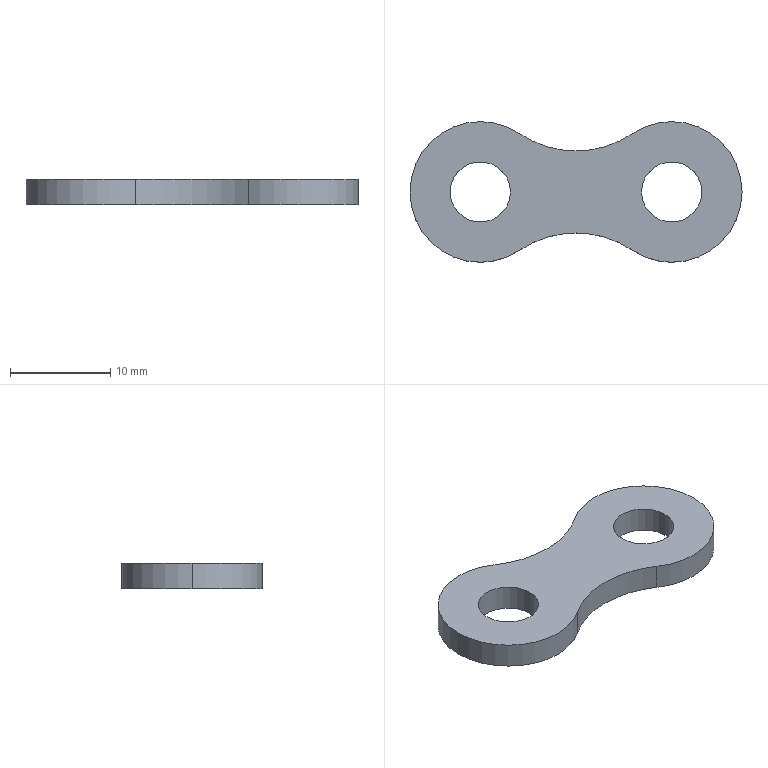Part | SolidWorks | features Extrusion 1 | 1 solid | 11 faces | box 33.05 x 14 x 2.55 mm | volume 777.67 mm3 | cylinder 9 | plane 2 | commonest cylinder face diameters 6 x4 14 x3 20 x2
STEP:
#1=CARTESIAN_POINT('',(16.05,0.,2.55));
#2=VERTEX_POINT('',#1);
#3=CARTESIAN_POINT('',(22.05,0.,2.55));
#4=VERTEX_POINT('',#3);
#5=CARTESIAN_POINT('',(19.05,0.,2.55));
#6=DIRECTION('',(0.,0.,1.));
#7=DIRECTION('',(1.,0.,0.));
#8=AXIS2_PLACEMENT_3D('',#5,#6,#7);
#9=CIRCLE('',#8,3.);
#10=EDGE_CURVE('',#2,#4,#9,.T.);
#11=ORIENTED_EDGE('',*,*,#10,.T.);
#12=CARTESIAN_POINT('',(22.05,0.,0.));
#13=VERTEX_POINT('',#12);
#14=CARTESIAN_POINT('',(22.05,0.,2.55));
#15=DIRECTION('',(0.,0.,-1.));
#16=VECTOR('',#15,1000.);
#17=LINE('',#14,#16);
#18=EDGE_CURVE('',#4,#13,#17,.T.);
#19=ORIENTED_EDGE('',*,*,#18,.T.);
#20=CARTESIAN_POINT('',(16.05,0.,0.));
#21=VERTEX_POINT('',#20);
#22=CARTESIAN_POINT('',(19.05,0.,0.));
#23=DIRECTION('',(0.,0.,1.));
#24=DIRECTION('',(1.,0.,0.));
#25=AXIS2_PLACEMENT_3D('',#22,#23,#24);
#26=CIRCLE('',#25,3.);
#27=EDGE_CURVE('',#21,#13,#26,.T.);
#28=ORIENTED_EDGE('',*,*,#27,.F.);
#29=CARTESIAN_POINT('',(16.05,0.,2.55));
#30=DIRECTION('',(0.,0.,-1.));
#31=VECTOR('',#30,1000.);
#32=LINE('',#29,#31);
#33=EDGE_CURVE('',#2,#21,#32,.T.);
#34=ORIENTED_EDGE('',*,*,#33,.F.);
#35=EDGE_LOOP('',(#11,#19,#28,#34));
#36=FACE_OUTER_BOUND('',#35,.T.);
#37=CARTESIAN_POINT('',(19.05,0.,2.55));
#38=DIRECTION('',(0.,0.,-1.));
#39=DIRECTION('',(-1.,0.,0.));
#40=AXIS2_PLACEMENT_3D('',#37,#38,#39);
#41=CYLINDRICAL_SURFACE('',#40,3.);
#42=ADVANCED_FACE('',(#36),#41,.F.);
#43=CARTESIAN_POINT('',(-3.,0.,2.55));
#44=VERTEX_POINT('',#43);
#45=CARTESIAN_POINT('',(3.,0.,2.55));
#46=VERTEX_POINT('',#45);
#47=CARTESIAN_POINT('',(0.,0.,2.55));
#48=DIRECTION('',(0.,0.,1.));
#49=DIRECTION('',(1.,0.,0.));
#50=AXIS2_PLACEMENT_3D('',#47,#48,#49);
#51=CIRCLE('',#50,3.);
#52=EDGE_CURVE('',#44,#46,#51,.T.);
#53=ORIENTED_EDGE('',*,*,#52,.T.);
#54=CARTESIAN_POINT('',(3.,0.,0.));
#55=VERTEX_POINT('',#54);
#56=CARTESIAN_POINT('',(3.,0.,2.55));
#57=DIRECTION('',(0.,0.,-1.));
#58=VECTOR('',#57,1000.);
#59=LINE('',#56,#58);
#60=EDGE_CURVE('',#46,#55,#59,.T.);
#61=ORIENTED_EDGE('',*,*,#60,.T.);
#62=CARTESIAN_POINT('',(-3.,0.,0.));
#63=VERTEX_POINT('',#62);
#64=CARTESIAN_POINT('',(0.,0.,0.));
#65=DIRECTION('',(0.,0.,1.));
#66=DIRECTION('',(1.,0.,0.));
#67=AXIS2_PLACEMENT_3D('',#64,#65,#66);
#68=CIRCLE('',#67,3.);
#69=EDGE_CURVE('',#63,#55,#68,.T.);
#70=ORIENTED_EDGE('',*,*,#69,.F.);
#71=CARTESIAN_POINT('',(-3.,0.,2.55));
#72=DIRECTION('',(0.,0.,-1.));
#73=VECTOR('',#72,1000.);
#74=LINE('',#71,#73);
#75=EDGE_CURVE('',#44,#63,#74,.T.);
#76=ORIENTED_EDGE('',*,*,#75,.F.);
#77=EDGE_LOOP('',(#53,#61,#70,#76));
#78=FACE_OUTER_BOUND('',#77,.T.);
#79=CARTESIAN_POINT('',(0.,0.,2.55));
#80=DIRECTION('',(0.,0.,-1.));
#81=DIRECTION('',(-1.,0.,0.));
#82=AXIS2_PLACEMENT_3D('',#79,#80,#81);
#83=CYLINDRICAL_SURFACE('',#82,3.);
#84=ADVANCED_FACE('',(#78),#83,.F.);
#85=CARTESIAN_POINT('',(-7.,0.,2.55));
#86=VERTEX_POINT('',#85);
#87=CARTESIAN_POINT('',(3.922,-5.798,2.55));
#88=VERTEX_POINT('',#87);
#89=CARTESIAN_POINT('',(0.,0.,2.55));
#90=DIRECTION('',(0.,0.,1.));
#91=DIRECTION('',(1.,0.,0.));
#92=AXIS2_PLACEMENT_3D('',#89,#90,#91);
#93=CIRCLE('',#92,7.);
#94=EDGE_CURVE('',#86,#88,#93,.T.);
#95=ORIENTED_EDGE('',*,*,#94,.F.);
#96=CARTESIAN_POINT('',(-7.,0.,0.));
#97=VERTEX_POINT('',#96);
#98=CARTESIAN_POINT('',(-7.,0.,2.55));
#99=DIRECTION('',(0.,0.,-1.));
#100=VECTOR('',#99,1000.);
#101=LINE('',#98,#100);
#102=EDGE_CURVE('',#86,#97,#101,.T.);
#103=ORIENTED_EDGE('',*,*,#102,.T.);
#104=CARTESIAN_POINT('',(3.922,-5.798,0.));
#105=VERTEX_POINT('',#104);
#106=CARTESIAN_POINT('',(0.,0.,0.));
#107=DIRECTION('',(0.,0.,1.));
#108=DIRECTION('',(1.,0.,0.));
#109=AXIS2_PLACEMENT_3D('',#106,#107,#108);
#110=CIRCLE('',#109,7.);
#111=EDGE_CURVE('',#97,#105,#110,.T.);
#112=ORIENTED_EDGE('',*,*,#111,.T.);
#113=CARTESIAN_POINT('',(3.922,-5.798,2.55));
#114=DIRECTION('',(0.,0.,-1.));
#115=VECTOR('',#114,1000.);
#116=LINE('',#113,#115);
#117=EDGE_CURVE('',#88,#105,#116,.T.);
#118=ORIENTED_EDGE('',*,*,#117,.F.);
#119=EDGE_LOOP('',(#95,#103,#112,#118));
#120=FACE_OUTER_BOUND('',#119,.T.);
#121=CARTESIAN_POINT('',(0.,0.,2.55));
#122=DIRECTION('',(0.,0.,-1.));
#123=DIRECTION('',(-1.,0.,0.));
#124=AXIS2_PLACEMENT_3D('',#121,#122,#123);
#125=CYLINDRICAL_SURFACE('',#124,7.);
#126=ADVANCED_FACE('',(#120),#125,.T.);
#127=ORIENTED_EDGE('',*,*,#52,.F.);
#128=CARTESIAN_POINT('',(0.,0.,2.55));
#129=DIRECTION('',(0.,0.,1.));
#130=DIRECTION('',(1.,0.,0.));
#131=AXIS2_PLACEMENT_3D('',#128,#129,#130);
#132=CIRCLE('',#131,3.);
#133=EDGE_CURVE('',#46,#44,#132,.T.);
#134=ORIENTED_EDGE('',*,*,#133,.F.);
#135=EDGE_LOOP('',(#127,#134));
#136=FACE_BOUND('',#135,.T.);
#137=CARTESIAN_POINT('',(15.128,5.798,2.55));
#138=VERTEX_POINT('',#137);
#139=CARTESIAN_POINT('',(3.922,5.798,2.55));
#140=VERTEX_POINT('',#139);
#141=CARTESIAN_POINT('',(9.525,14.081,2.55));
#142=DIRECTION('',(0.,0.,-1.));
#143=DIRECTION('',(1.,0.,0.));
#144=AXIS2_PLACEMENT_3D('',#141,#142,#143);
#145=CIRCLE('',#144,10.);
#146=EDGE_CURVE('',#138,#140,#145,.T.);
#147=ORIENTED_EDGE('',*,*,#146,.T.);
#148=CARTESIAN_POINT('',(0.,0.,2.55));
#149=DIRECTION('',(0.,0.,1.));
#150=DIRECTION('',(1.,0.,0.));
#151=AXIS2_PLACEMENT_3D('',#148,#149,#150);
#152=CIRCLE('',#151,7.);
#153=EDGE_CURVE('',#140,#86,#152,.T.);
#154=ORIENTED_EDGE('',*,*,#153,.T.);
#155=ORIENTED_EDGE('',*,*,#94,.T.);
#156=CARTESIAN_POINT('',(15.128,-5.798,2.55));
#157=VERTEX_POINT('',#156);
#158=CARTESIAN_POINT('',(9.525,-14.081,2.55));
#159=DIRECTION('',(0.,0.,-1.));
#160=DIRECTION('',(-1.,0.,0.));
#161=AXIS2_PLACEMENT_3D('',#158,#159,#160);
#162=CIRCLE('',#161,10.);
#163=EDGE_CURVE('',#88,#157,#162,.T.);
#164=ORIENTED_EDGE('',*,*,#163,.T.);
#165=CARTESIAN_POINT('',(19.05,0.,2.55));
#166=DIRECTION('',(0.,0.,1.));
#167=DIRECTION('',(1.,0.,0.));
#168=AXIS2_PLACEMENT_3D('',#165,#166,#167);
#169=CIRCLE('',#168,7.);
#170=EDGE_CURVE('',#157,#138,#169,.T.);
#171=ORIENTED_EDGE('',*,*,#170,.T.);
#172=EDGE_LOOP('',(#147,#154,#155,#164,#171));
#173=FACE_OUTER_BOUND('',#172,.T.);
#174=ORIENTED_EDGE('',*,*,#10,.F.);
#175=CARTESIAN_POINT('',(19.05,0.,2.55));
#176=DIRECTION('',(0.,0.,1.));
#177=DIRECTION('',(1.,0.,0.));
#178=AXIS2_PLACEMENT_3D('',#175,#176,#177);
#179=CIRCLE('',#178,3.);
#180=EDGE_CURVE('',#4,#2,#179,.T.);
#181=ORIENTED_EDGE('',*,*,#180,.F.);
#182=EDGE_LOOP('',(#174,#181));
#183=FACE_BOUND('',#182,.T.);
#184=CARTESIAN_POINT('',(14.288,7.04,2.55));
#185=DIRECTION('',(0.,0.,1.));
#186=DIRECTION('',(1.,0.,0.));
#187=AXIS2_PLACEMENT_3D('',#184,#185,#186);
#188=PLANE('',#187);
#189=ADVANCED_FACE('',(#136,#173,#183),#188,.T.);
#190=ORIENTED_EDGE('',*,*,#69,.T.);
#191=CARTESIAN_POINT('',(0.,0.,0.));
#192=DIRECTION('',(0.,0.,1.));
#193=DIRECTION('',(1.,0.,0.));
#194=AXIS2_PLACEMENT_3D('',#191,#192,#193);
#195=CIRCLE('',#194,3.);
#196=EDGE_CURVE('',#55,#63,#195,.T.);
#197=ORIENTED_EDGE('',*,*,#196,.T.);
#198=EDGE_LOOP('',(#190,#197));
#199=FACE_BOUND('',#198,.T.);
#200=CARTESIAN_POINT('',(15.128,5.798,0.));
#201=VERTEX_POINT('',#200);
#202=CARTESIAN_POINT('',(3.922,5.798,0.));
#203=VERTEX_POINT('',#202);
#204=CARTESIAN_POINT('',(9.525,14.081,0.));
#205=DIRECTION('',(0.,0.,-1.));
#206=DIRECTION('',(1.,0.,0.));
#207=AXIS2_PLACEMENT_3D('',#204,#205,#206);
#208=CIRCLE('',#207,10.);
#209=EDGE_CURVE('',#201,#203,#208,.T.);
#210=ORIENTED_EDGE('',*,*,#209,.F.);
#211=CARTESIAN_POINT('',(15.128,-5.798,0.));
#212=VERTEX_POINT('',#211);
#213=CARTESIAN_POINT('',(19.05,0.,0.));
#214=DIRECTION('',(0.,0.,1.));
#215=DIRECTION('',(1.,0.,0.));
#216=AXIS2_PLACEMENT_3D('',#213,#214,#215);
#217=CIRCLE('',#216,7.);
#218=EDGE_CURVE('',#212,#201,#217,.T.);
#219=ORIENTED_EDGE('',*,*,#218,.F.);
#220=CARTESIAN_POINT('',(9.525,-14.081,0.));
#221=DIRECTION('',(0.,0.,-1.));
#222=DIRECTION('',(-1.,0.,0.));
#223=AXIS2_PLACEMENT_3D('',#220,#221,#222);
#224=CIRCLE('',#223,10.);
#225=EDGE_CURVE('',#105,#212,#224,.T.);
#226=ORIENTED_EDGE('',*,*,#225,.F.);
#227=ORIENTED_EDGE('',*,*,#111,.F.);
#228=CARTESIAN_POINT('',(0.,0.,0.));
#229=DIRECTION('',(0.,0.,1.));
#230=DIRECTION('',(1.,0.,0.));
#231=AXIS2_PLACEMENT_3D('',#228,#229,#230);
#232=CIRCLE('',#231,7.);
#233=EDGE_CURVE('',#203,#97,#232,.T.);
#234=ORIENTED_EDGE('',*,*,#233,.F.);
#235=EDGE_LOOP('',(#210,#219,#226,#227,#234));
#236=FACE_OUTER_BOUND('',#235,.T.);
#237=ORIENTED_EDGE('',*,*,#27,.T.);
#238=CARTESIAN_POINT('',(19.05,0.,0.));
#239=DIRECTION('',(0.,0.,1.));
#240=DIRECTION('',(1.,0.,0.));
#241=AXIS2_PLACEMENT_3D('',#238,#239,#240);
#242=CIRCLE('',#241,3.);
#243=EDGE_CURVE('',#13,#21,#242,.T.);
#244=ORIENTED_EDGE('',*,*,#243,.T.);
#245=EDGE_LOOP('',(#237,#244));
#246=FACE_BOUND('',#245,.T.);
#247=CARTESIAN_POINT('',(14.288,7.04,0.));
#248=DIRECTION('',(0.,0.,1.));
#249=DIRECTION('',(1.,0.,0.));
#250=AXIS2_PLACEMENT_3D('',#247,#248,#249);
#251=PLANE('',#250);
#252=ADVANCED_FACE('',(#199,#236,#246),#251,.F.);
#253=ORIENTED_EDGE('',*,*,#209,.T.);
#254=CARTESIAN_POINT('',(3.922,5.798,2.55));
#255=DIRECTION('',(0.,0.,-1.));
#256=VECTOR('',#255,1000.);
#257=LINE('',#254,#256);
#258=EDGE_CURVE('',#140,#203,#257,.T.);
#259=ORIENTED_EDGE('',*,*,#258,.F.);
#260=ORIENTED_EDGE('',*,*,#146,.F.);
#261=CARTESIAN_POINT('',(15.128,5.798,2.55));
#262=DIRECTION('',(0.,0.,-1.));
#263=VECTOR('',#262,1000.);
#264=LINE('',#261,#263);
#265=EDGE_CURVE('',#138,#201,#264,.T.);
#266=ORIENTED_EDGE('',*,*,#265,.T.);
#267=EDGE_LOOP('',(#253,#259,#260,#266));
#268=FACE_OUTER_BOUND('',#267,.T.);
#269=CARTESIAN_POINT('',(9.525,14.081,2.55));
#270=DIRECTION('',(0.,0.,-1.));
#271=DIRECTION('',(-1.,0.,0.));
#272=AXIS2_PLACEMENT_3D('',#269,#270,#271);
#273=CYLINDRICAL_SURFACE('',#272,10.);
#274=ADVANCED_FACE('',(#268),#273,.F.);
#275=ORIENTED_EDGE('',*,*,#102,.F.);
#276=ORIENTED_EDGE('',*,*,#153,.F.);
#277=ORIENTED_EDGE('',*,*,#258,.T.);
#278=ORIENTED_EDGE('',*,*,#233,.T.);
#279=EDGE_LOOP('',(#275,#276,#277,#278));
#280=FACE_OUTER_BOUND('',#279,.T.);
#281=CARTESIAN_POINT('',(0.,0.,2.55));
#282=DIRECTION('',(0.,0.,-1.));
#283=DIRECTION('',(-1.,0.,0.));
#284=AXIS2_PLACEMENT_3D('',#281,#282,#283);
#285=CYLINDRICAL_SURFACE('',#284,7.);
#286=ADVANCED_FACE('',(#280),#285,.T.);
#287=ORIENTED_EDGE('',*,*,#225,.T.);
#288=CARTESIAN_POINT('',(15.128,-5.798,2.55));
#289=DIRECTION('',(0.,0.,-1.));
#290=VECTOR('',#289,1000.);
#291=LINE('',#288,#290);
#292=EDGE_CURVE('',#157,#212,#291,.T.);
#293=ORIENTED_EDGE('',*,*,#292,.F.);
#294=ORIENTED_EDGE('',*,*,#163,.F.);
#295=ORIENTED_EDGE('',*,*,#117,.T.);
#296=EDGE_LOOP('',(#287,#293,#294,#295));
#297=FACE_OUTER_BOUND('',#296,.T.);
#298=CARTESIAN_POINT('',(9.525,-14.081,2.55));
#299=DIRECTION('',(0.,0.,-1.));
#300=DIRECTION('',(-1.,0.,0.));
#301=AXIS2_PLACEMENT_3D('',#298,#299,#300);
#302=CYLINDRICAL_SURFACE('',#301,10.);
#303=ADVANCED_FACE('',(#297),#302,.F.);
#304=ORIENTED_EDGE('',*,*,#218,.T.);
#305=ORIENTED_EDGE('',*,*,#265,.F.);
#306=ORIENTED_EDGE('',*,*,#170,.F.);
#307=ORIENTED_EDGE('',*,*,#292,.T.);
#308=EDGE_LOOP('',(#304,#305,#306,#307));
#309=FACE_OUTER_BOUND('',#308,.T.);
#310=CARTESIAN_POINT('',(19.05,0.,2.55));
#311=DIRECTION('',(0.,0.,-1.));
#312=DIRECTION('',(-1.,0.,0.));
#313=AXIS2_PLACEMENT_3D('',#310,#311,#312);
#314=CYLINDRICAL_SURFACE('',#313,7.);
#315=ADVANCED_FACE('',(#309),#314,.T.);
#316=ORIENTED_EDGE('',*,*,#60,.F.);
#317=ORIENTED_EDGE('',*,*,#133,.T.);
#318=ORIENTED_EDGE('',*,*,#75,.T.);
#319=ORIENTED_EDGE('',*,*,#196,.F.);
#320=EDGE_LOOP('',(#316,#317,#318,#319));
#321=FACE_OUTER_BOUND('',#320,.T.);
#322=CARTESIAN_POINT('',(0.,0.,2.55));
#323=DIRECTION('',(0.,0.,-1.));
#324=DIRECTION('',(-1.,0.,0.));
#325=AXIS2_PLACEMENT_3D('',#322,#323,#324);
#326=CYLINDRICAL_SURFACE('',#325,3.);
#327=ADVANCED_FACE('',(#321),#326,.F.);
#328=ORIENTED_EDGE('',*,*,#18,.F.);
#329=ORIENTED_EDGE('',*,*,#180,.T.);
#330=ORIENTED_EDGE('',*,*,#33,.T.);
#331=ORIENTED_EDGE('',*,*,#243,.F.);
#332=EDGE_LOOP('',(#328,#329,#330,#331));
#333=FACE_OUTER_BOUND('',#332,.T.);
#334=CARTESIAN_POINT('',(19.05,0.,2.55));
#335=DIRECTION('',(0.,0.,-1.));
#336=DIRECTION('',(-1.,0.,0.));
#337=AXIS2_PLACEMENT_3D('',#334,#335,#336);
#338=CYLINDRICAL_SURFACE('',#337,3.);
#339=ADVANCED_FACE('',(#333),#338,.F.);
#340=CLOSED_SHELL('',(#42,#84,#126,#189,#252,#274,#286,#303,#315,#327,#339));
#341=MANIFOLD_SOLID_BREP('',#340);
#342=CARTESIAN_POINT('',(0.,0.,0.));
#343=DIRECTION('',(0.,0.,1.));
#344=DIRECTION('',(1.,0.,0.));
#345=AXIS2_PLACEMENT_3D('',#342,#343,#344);
#346=(LENGTH_UNIT()NAMED_UNIT(*)SI_UNIT(.MILLI.,.METRE.));
#347=UNCERTAINTY_MEASURE_WITH_UNIT(LENGTH_MEASURE(0.00001),#346,'','');
#348=(NAMED_UNIT(*)PLANE_ANGLE_UNIT()SI_UNIT($,.RADIAN.));
#349=(NAMED_UNIT(*)SI_UNIT($,.STERADIAN.)SOLID_ANGLE_UNIT());
#350=(GEOMETRIC_REPRESENTATION_CONTEXT(3)GLOBAL_UNCERTAINTY_ASSIGNED_CONTEXT((#347))GLOBAL_UNIT_ASSIGNED_CONTEXT((#346,#348,#349))REPRESENTATION_CONTEXT('',''));
#351=ADVANCED_BREP_SHAPE_REPRESENTATION('',(#341,#345),#350);